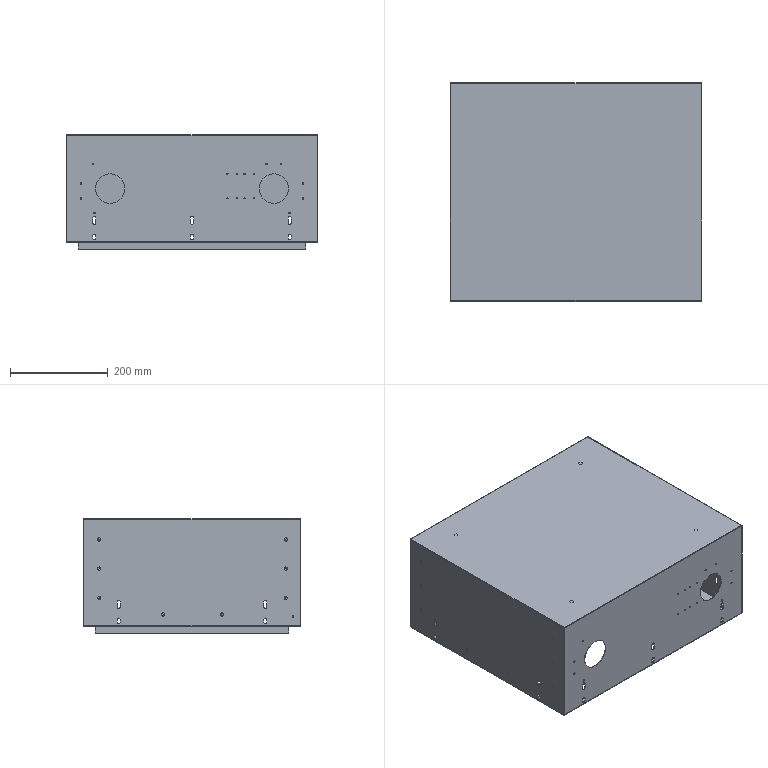Part | STEP file | 1 solid | 470 faces | box 515 x 446 x 234 mm | volume 856637 mm3 | cylinder 230 | plane 196 | cone 40 | spline 4 | commonest cylinder face diameters 3.3 x66 6.2 x60 7 x40 2.5 x16 0.02 x12 2.42 x12